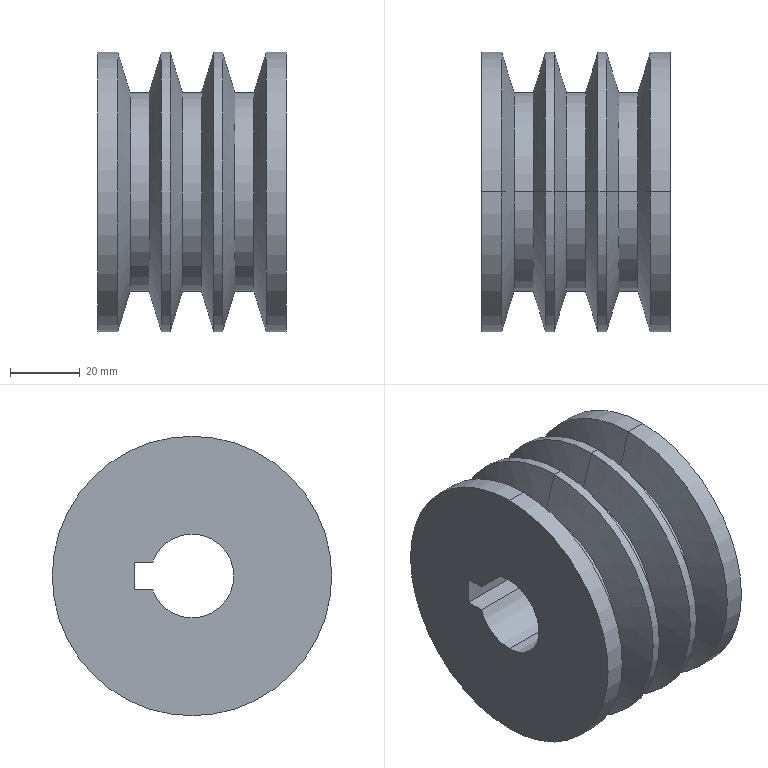Part | STEP file | Motor pulley | 1 solid | 37 faces | box 54 x 80 x 80 mm | volume 176576 mm3 | cylinder 19 | cone 12 | plane 6 | commonest cylinder face diameters 80 x8 57 x6 24 x3 2.8 x2
STEP:
#1=CARTESIAN_POINT('',(52.,-16.,1.4));
#2=VERTEX_POINT('',#1);
#3=CARTESIAN_POINT('',(52.,-16.,-1.4));
#4=VERTEX_POINT('',#3);
#5=CARTESIAN_POINT('',(52.,-16.,0.));
#6=DIRECTION('',(1.,0.,0.));
#7=DIRECTION('',(0.,0.,-1.));
#8=AXIS2_PLACEMENT_3D('',#5,#6,#7);
#9=CIRCLE('',#8,1.4);
#10=EDGE_CURVE('',#2,#4,#9,.T.);
#11=ORIENTED_EDGE('',*,*,#10,.F.);
#12=CARTESIAN_POINT('',(54.,-16.,1.4));
#13=VERTEX_POINT('',#12);
#14=CARTESIAN_POINT('',(52.,-16.,1.4));
#15=DIRECTION('',(1.,0.,0.));
#16=VECTOR('',#15,1000.);
#17=LINE('',#14,#16);
#18=EDGE_CURVE('',#2,#13,#17,.T.);
#19=ORIENTED_EDGE('',*,*,#18,.T.);
#20=CARTESIAN_POINT('',(54.,-16.,-1.4));
#21=VERTEX_POINT('',#20);
#22=CARTESIAN_POINT('',(54.,-16.,0.));
#23=DIRECTION('',(1.,0.,0.));
#24=DIRECTION('',(0.,0.,-1.));
#25=AXIS2_PLACEMENT_3D('',#22,#23,#24);
#26=CIRCLE('',#25,1.4);
#27=EDGE_CURVE('',#13,#21,#26,.T.);
#28=ORIENTED_EDGE('',*,*,#27,.T.);
#29=CARTESIAN_POINT('',(52.,-16.,-1.4));
#30=DIRECTION('',(1.,0.,0.));
#31=VECTOR('',#30,1000.);
#32=LINE('',#29,#31);
#33=EDGE_CURVE('',#4,#21,#32,.T.);
#34=ORIENTED_EDGE('',*,*,#33,.F.);
#35=EDGE_LOOP('',(#11,#19,#28,#34));
#36=FACE_OUTER_BOUND('',#35,.T.);
#37=CARTESIAN_POINT('',(52.,-16.,0.));
#38=DIRECTION('',(1.,0.,0.));
#39=DIRECTION('',(0.,0.,-1.));
#40=AXIS2_PLACEMENT_3D('',#37,#38,#39);
#41=CYLINDRICAL_SURFACE('',#40,1.4);
#42=ADVANCED_FACE('',(#36),#41,.F.);
#43=CARTESIAN_POINT('',(54.,0.,-12.));
#44=VERTEX_POINT('',#43);
#45=CARTESIAN_POINT('',(54.,0.,12.));
#46=VERTEX_POINT('',#45);
#47=CARTESIAN_POINT('',(54.,0.,0.));
#48=DIRECTION('',(-1.,0.,0.));
#49=DIRECTION('',(0.,0.,1.));
#50=AXIS2_PLACEMENT_3D('',#47,#48,#49);
#51=CIRCLE('',#50,12.);
#52=EDGE_CURVE('',#44,#46,#51,.T.);
#53=ORIENTED_EDGE('',*,*,#52,.F.);
#54=CARTESIAN_POINT('',(0.,0.,-12.));
#55=VERTEX_POINT('',#54);
#56=CARTESIAN_POINT('',(55.,0.,-12.));
#57=DIRECTION('',(-1.,0.,0.));
#58=VECTOR('',#57,1000.);
#59=LINE('',#56,#58);
#60=EDGE_CURVE('',#44,#55,#59,.T.);
#61=ORIENTED_EDGE('',*,*,#60,.T.);
#62=CARTESIAN_POINT('',(0.,0.,12.));
#63=VERTEX_POINT('',#62);
#64=CARTESIAN_POINT('',(0.,0.,0.));
#65=DIRECTION('',(-1.,0.,0.));
#66=DIRECTION('',(0.,0.,1.));
#67=AXIS2_PLACEMENT_3D('',#64,#65,#66);
#68=CIRCLE('',#67,12.);
#69=EDGE_CURVE('',#55,#63,#68,.T.);
#70=ORIENTED_EDGE('',*,*,#69,.T.);
#71=CARTESIAN_POINT('',(55.,0.,12.));
#72=DIRECTION('',(-1.,0.,0.));
#73=VECTOR('',#72,1000.);
#74=LINE('',#71,#73);
#75=EDGE_CURVE('',#46,#63,#74,.T.);
#76=ORIENTED_EDGE('',*,*,#75,.F.);
#77=EDGE_LOOP('',(#53,#61,#70,#76));
#78=FACE_OUTER_BOUND('',#77,.T.);
#79=CARTESIAN_POINT('',(55.,0.,0.));
#80=DIRECTION('',(-1.,0.,0.));
#81=DIRECTION('',(0.,0.,1.));
#82=AXIS2_PLACEMENT_3D('',#79,#80,#81);
#83=CYLINDRICAL_SURFACE('',#82,12.);
#84=ADVANCED_FACE('',(#78),#83,.F.);
#85=CARTESIAN_POINT('',(54.,11.314,4.));
#86=VERTEX_POINT('',#85);
#87=CARTESIAN_POINT('',(54.,0.,0.));
#88=DIRECTION('',(-1.,0.,0.));
#89=DIRECTION('',(0.,0.,1.));
#90=AXIS2_PLACEMENT_3D('',#87,#88,#89);
#91=CIRCLE('',#90,12.);
#92=EDGE_CURVE('',#46,#86,#91,.T.);
#93=ORIENTED_EDGE('',*,*,#92,.F.);
#94=ORIENTED_EDGE('',*,*,#75,.T.);
#95=CARTESIAN_POINT('',(0.,11.314,4.));
#96=VERTEX_POINT('',#95);
#97=CARTESIAN_POINT('',(0.,0.,0.));
#98=DIRECTION('',(-1.,0.,0.));
#99=DIRECTION('',(0.,0.,1.));
#100=AXIS2_PLACEMENT_3D('',#97,#98,#99);
#101=CIRCLE('',#100,12.);
#102=EDGE_CURVE('',#63,#96,#101,.T.);
#103=ORIENTED_EDGE('',*,*,#102,.T.);
#104=CARTESIAN_POINT('',(55.,11.314,4.));
#105=DIRECTION('',(1.,0.,0.));
#106=VECTOR('',#105,1000.);
#107=LINE('',#104,#106);
#108=EDGE_CURVE('',#96,#86,#107,.T.);
#109=ORIENTED_EDGE('',*,*,#108,.T.);
#110=EDGE_LOOP('',(#93,#94,#103,#109));
#111=FACE_OUTER_BOUND('',#110,.T.);
#112=CARTESIAN_POINT('',(55.,0.,0.));
#113=DIRECTION('',(-1.,0.,0.));
#114=DIRECTION('',(0.,0.,1.));
#115=AXIS2_PLACEMENT_3D('',#112,#113,#114);
#116=CYLINDRICAL_SURFACE('',#115,12.);
#117=ADVANCED_FACE('',(#111),#116,.F.);
#118=CARTESIAN_POINT('',(54.,0.,40.));
#119=VERTEX_POINT('',#118);
#120=CARTESIAN_POINT('',(54.,0.,-40.));
#121=VERTEX_POINT('',#120);
#122=CARTESIAN_POINT('',(54.,0.,0.));
#123=DIRECTION('',(-1.,0.,0.));
#124=DIRECTION('',(0.,0.,1.));
#125=AXIS2_PLACEMENT_3D('',#122,#123,#124);
#126=CIRCLE('',#125,40.);
#127=EDGE_CURVE('',#119,#121,#126,.T.);
#128=ORIENTED_EDGE('',*,*,#127,.T.);
#129=CARTESIAN_POINT('',(48.264,0.,-40.));
#130=VERTEX_POINT('',#129);
#131=CARTESIAN_POINT('',(0.,0.,-40.));
#132=DIRECTION('',(-1.,0.,0.));
#133=VECTOR('',#132,1000.);
#134=LINE('',#131,#133);
#135=EDGE_CURVE('',#121,#130,#134,.T.);
#136=ORIENTED_EDGE('',*,*,#135,.T.);
#137=CARTESIAN_POINT('',(48.264,0.,40.));
#138=VERTEX_POINT('',#137);
#139=CARTESIAN_POINT('',(48.264,0.,0.));
#140=DIRECTION('',(-1.,0.,0.));
#141=DIRECTION('',(0.,0.,1.));
#142=AXIS2_PLACEMENT_3D('',#139,#140,#141);
#143=CIRCLE('',#142,40.);
#144=EDGE_CURVE('',#138,#130,#143,.T.);
#145=ORIENTED_EDGE('',*,*,#144,.F.);
#146=CARTESIAN_POINT('',(0.,0.,40.));
#147=DIRECTION('',(-1.,0.,0.));
#148=VECTOR('',#147,1000.);
#149=LINE('',#146,#148);
#150=EDGE_CURVE('',#119,#138,#149,.T.);
#151=ORIENTED_EDGE('',*,*,#150,.F.);
#152=EDGE_LOOP('',(#128,#136,#145,#151));
#153=FACE_OUTER_BOUND('',#152,.T.);
#154=CARTESIAN_POINT('',(0.,0.,0.));
#155=DIRECTION('',(-1.,0.,0.));
#156=DIRECTION('',(0.,0.,1.));
#157=AXIS2_PLACEMENT_3D('',#154,#155,#156);
#158=CYLINDRICAL_SURFACE('',#157,40.);
#159=ADVANCED_FACE('',(#153),#158,.T.);
#160=CARTESIAN_POINT('',(44.748,0.,28.5));
#161=VERTEX_POINT('',#160);
#162=CARTESIAN_POINT('',(44.748,0.,-28.5));
#163=VERTEX_POINT('',#162);
#164=CARTESIAN_POINT('',(44.748,0.,0.));
#165=DIRECTION('',(-1.,0.,0.));
#166=DIRECTION('',(0.,0.,1.));
#167=AXIS2_PLACEMENT_3D('',#164,#165,#166);
#168=CIRCLE('',#167,28.5);
#169=EDGE_CURVE('',#161,#163,#168,.T.);
#170=ORIENTED_EDGE('',*,*,#169,.F.);
#171=CARTESIAN_POINT('',(48.264,0.,40.));
#172=DIRECTION('',(0.2924,0.,0.9563));
#173=VECTOR('',#172,1000.);
#174=LINE('',#171,#173);
#175=EDGE_CURVE('',#161,#138,#174,.T.);
#176=ORIENTED_EDGE('',*,*,#175,.T.);
#177=ORIENTED_EDGE('',*,*,#144,.T.);
#178=CARTESIAN_POINT('',(48.264,0.,-40.));
#179=DIRECTION('',(0.2924,0.,-0.9563));
#180=VECTOR('',#179,1000.);
#181=LINE('',#178,#180);
#182=EDGE_CURVE('',#163,#130,#181,.T.);
#183=ORIENTED_EDGE('',*,*,#182,.F.);
#184=EDGE_LOOP('',(#170,#176,#177,#183));
#185=FACE_OUTER_BOUND('',#184,.T.);
#186=CARTESIAN_POINT('',(48.264,0.,0.));
#187=DIRECTION('',(1.,0.,0.));
#188=DIRECTION('',(0.,0.,-1.));
#189=AXIS2_PLACEMENT_3D('',#186,#187,#188);
#190=CONICAL_SURFACE('',#189,40.,1.274);
#191=ADVANCED_FACE('',(#185),#190,.T.);
#192=ORIENTED_EDGE('',*,*,#169,.T.);
#193=CARTESIAN_POINT('',(39.252,0.,-28.5));
#194=VERTEX_POINT('',#193);
#195=CARTESIAN_POINT('',(0.,0.,-28.5));
#196=DIRECTION('',(-1.,0.,0.));
#197=VECTOR('',#196,1000.);
#198=LINE('',#195,#197);
#199=EDGE_CURVE('',#163,#194,#198,.T.);
#200=ORIENTED_EDGE('',*,*,#199,.T.);
#201=CARTESIAN_POINT('',(39.252,0.,28.5));
#202=VERTEX_POINT('',#201);
#203=CARTESIAN_POINT('',(39.252,0.,0.));
#204=DIRECTION('',(-1.,0.,0.));
#205=DIRECTION('',(0.,0.,1.));
#206=AXIS2_PLACEMENT_3D('',#203,#204,#205);
#207=CIRCLE('',#206,28.5);
#208=EDGE_CURVE('',#202,#194,#207,.T.);
#209=ORIENTED_EDGE('',*,*,#208,.F.);
#210=CARTESIAN_POINT('',(0.,0.,28.5));
#211=DIRECTION('',(-1.,0.,0.));
#212=VECTOR('',#211,1000.);
#213=LINE('',#210,#212);
#214=EDGE_CURVE('',#161,#202,#213,.T.);
#215=ORIENTED_EDGE('',*,*,#214,.F.);
#216=EDGE_LOOP('',(#192,#200,#209,#215));
#217=FACE_OUTER_BOUND('',#216,.T.);
#218=CARTESIAN_POINT('',(0.,0.,0.));
#219=DIRECTION('',(-1.,0.,0.));
#220=DIRECTION('',(0.,0.,1.));
#221=AXIS2_PLACEMENT_3D('',#218,#219,#220);
#222=CYLINDRICAL_SURFACE('',#221,28.5);
#223=ADVANCED_FACE('',(#217),#222,.T.);
#224=ORIENTED_EDGE('',*,*,#208,.T.);
#225=CARTESIAN_POINT('',(35.736,0.,-40.));
#226=VERTEX_POINT('',#225);
#227=CARTESIAN_POINT('',(39.252,0.,-28.5));
#228=DIRECTION('',(-0.2924,0.,-0.9563));
#229=VECTOR('',#228,1000.);
#230=LINE('',#227,#229);
#231=EDGE_CURVE('',#194,#226,#230,.T.);
#232=ORIENTED_EDGE('',*,*,#231,.T.);
#233=CARTESIAN_POINT('',(35.736,0.,40.));
#234=VERTEX_POINT('',#233);
#235=CARTESIAN_POINT('',(35.736,0.,0.));
#236=DIRECTION('',(-1.,0.,0.));
#237=DIRECTION('',(0.,0.,1.));
#238=AXIS2_PLACEMENT_3D('',#235,#236,#237);
#239=CIRCLE('',#238,40.);
#240=EDGE_CURVE('',#234,#226,#239,.T.);
#241=ORIENTED_EDGE('',*,*,#240,.F.);
#242=CARTESIAN_POINT('',(39.252,0.,28.5));
#243=DIRECTION('',(-0.2924,0.,0.9563));
#244=VECTOR('',#243,1000.);
#245=LINE('',#242,#244);
#246=EDGE_CURVE('',#202,#234,#245,.T.);
#247=ORIENTED_EDGE('',*,*,#246,.F.);
#248=EDGE_LOOP('',(#224,#232,#241,#247));
#249=FACE_OUTER_BOUND('',#248,.T.);
#250=CARTESIAN_POINT('',(39.252,0.,0.));
#251=DIRECTION('',(-1.,0.,0.));
#252=DIRECTION('',(0.,0.,1.));
#253=AXIS2_PLACEMENT_3D('',#250,#251,#252);
#254=CONICAL_SURFACE('',#253,28.5,1.274);
#255=ADVANCED_FACE('',(#249),#254,.T.);
#256=ORIENTED_EDGE('',*,*,#240,.T.);
#257=CARTESIAN_POINT('',(33.264,0.,-40.));
#258=VERTEX_POINT('',#257);
#259=CARTESIAN_POINT('',(0.,0.,-40.));
#260=DIRECTION('',(-1.,0.,0.));
#261=VECTOR('',#260,1000.);
#262=LINE('',#259,#261);
#263=EDGE_CURVE('',#226,#258,#262,.T.);
#264=ORIENTED_EDGE('',*,*,#263,.T.);
#265=CARTESIAN_POINT('',(33.264,0.,40.));
#266=VERTEX_POINT('',#265);
#267=CARTESIAN_POINT('',(33.264,0.,0.));
#268=DIRECTION('',(-1.,0.,0.));
#269=DIRECTION('',(0.,0.,1.));
#270=AXIS2_PLACEMENT_3D('',#267,#268,#269);
#271=CIRCLE('',#270,40.);
#272=EDGE_CURVE('',#266,#258,#271,.T.);
#273=ORIENTED_EDGE('',*,*,#272,.F.);
#274=CARTESIAN_POINT('',(0.,0.,40.));
#275=DIRECTION('',(-1.,0.,0.));
#276=VECTOR('',#275,1000.);
#277=LINE('',#274,#276);
#278=EDGE_CURVE('',#234,#266,#277,.T.);
#279=ORIENTED_EDGE('',*,*,#278,.F.);
#280=EDGE_LOOP('',(#256,#264,#273,#279));
#281=FACE_OUTER_BOUND('',#280,.T.);
#282=CARTESIAN_POINT('',(0.,0.,0.));
#283=DIRECTION('',(-1.,0.,0.));
#284=DIRECTION('',(0.,0.,1.));
#285=AXIS2_PLACEMENT_3D('',#282,#283,#284);
#286=CYLINDRICAL_SURFACE('',#285,40.);
#287=ADVANCED_FACE('',(#281),#286,.T.);
#288=CARTESIAN_POINT('',(29.748,0.,28.5));
#289=VERTEX_POINT('',#288);
#290=CARTESIAN_POINT('',(29.748,0.,-28.5));
#291=VERTEX_POINT('',#290);
#292=CARTESIAN_POINT('',(29.748,0.,0.));
#293=DIRECTION('',(-1.,0.,0.));
#294=DIRECTION('',(0.,0.,1.));
#295=AXIS2_PLACEMENT_3D('',#292,#293,#294);
#296=CIRCLE('',#295,28.5);
#297=EDGE_CURVE('',#289,#291,#296,.T.);
#298=ORIENTED_EDGE('',*,*,#297,.F.);
#299=CARTESIAN_POINT('',(33.264,0.,40.));
#300=DIRECTION('',(0.2924,0.,0.9563));
#301=VECTOR('',#300,1000.);
#302=LINE('',#299,#301);
#303=EDGE_CURVE('',#289,#266,#302,.T.);
#304=ORIENTED_EDGE('',*,*,#303,.T.);
#305=ORIENTED_EDGE('',*,*,#272,.T.);
#306=CARTESIAN_POINT('',(33.264,0.,-40.));
#307=DIRECTION('',(0.2924,0.,-0.9563));
#308=VECTOR('',#307,1000.);
#309=LINE('',#306,#308);
#310=EDGE_CURVE('',#291,#258,#309,.T.);
#311=ORIENTED_EDGE('',*,*,#310,.F.);
#312=EDGE_LOOP('',(#298,#304,#305,#311));
#313=FACE_OUTER_BOUND('',#312,.T.);
#314=CARTESIAN_POINT('',(33.264,0.,0.));
#315=DIRECTION('',(1.,0.,0.));
#316=DIRECTION('',(0.,0.,-1.));
#317=AXIS2_PLACEMENT_3D('',#314,#315,#316);
#318=CONICAL_SURFACE('',#317,40.,1.274);
#319=ADVANCED_FACE('',(#313),#318,.T.);
#320=ORIENTED_EDGE('',*,*,#297,.T.);
#321=CARTESIAN_POINT('',(24.252,0.,-28.5));
#322=VERTEX_POINT('',#321);
#323=CARTESIAN_POINT('',(0.,0.,-28.5));
#324=DIRECTION('',(-1.,0.,0.));
#325=VECTOR('',#324,1000.);
#326=LINE('',#323,#325);
#327=EDGE_CURVE('',#291,#322,#326,.T.);
#328=ORIENTED_EDGE('',*,*,#327,.T.);
#329=CARTESIAN_POINT('',(24.252,0.,28.5));
#330=VERTEX_POINT('',#329);
#331=CARTESIAN_POINT('',(24.252,0.,0.));
#332=DIRECTION('',(-1.,0.,0.));
#333=DIRECTION('',(0.,0.,1.));
#334=AXIS2_PLACEMENT_3D('',#331,#332,#333);
#335=CIRCLE('',#334,28.5);
#336=EDGE_CURVE('',#330,#322,#335,.T.);
#337=ORIENTED_EDGE('',*,*,#336,.F.);
#338=CARTESIAN_POINT('',(0.,0.,28.5));
#339=DIRECTION('',(-1.,0.,0.));
#340=VECTOR('',#339,1000.);
#341=LINE('',#338,#340);
#342=EDGE_CURVE('',#289,#330,#341,.T.);
#343=ORIENTED_EDGE('',*,*,#342,.F.);
#344=EDGE_LOOP('',(#320,#328,#337,#343));
#345=FACE_OUTER_BOUND('',#344,.T.);
#346=CARTESIAN_POINT('',(0.,0.,0.));
#347=DIRECTION('',(-1.,0.,0.));
#348=DIRECTION('',(0.,0.,1.));
#349=AXIS2_PLACEMENT_3D('',#346,#347,#348);
#350=CYLINDRICAL_SURFACE('',#349,28.5);
#351=ADVANCED_FACE('',(#345),#350,.T.);
#352=ORIENTED_EDGE('',*,*,#336,.T.);
#353=CARTESIAN_POINT('',(20.736,0.,-40.));
#354=VERTEX_POINT('',#353);
#355=CARTESIAN_POINT('',(24.252,0.,-28.5));
#356=DIRECTION('',(-0.2924,0.,-0.9563));
#357=VECTOR('',#356,1000.);
#358=LINE('',#355,#357);
#359=EDGE_CURVE('',#322,#354,#358,.T.);
#360=ORIENTED_EDGE('',*,*,#359,.T.);
#361=CARTESIAN_POINT('',(20.736,0.,40.));
#362=VERTEX_POINT('',#361);
#363=CARTESIAN_POINT('',(20.736,0.,0.));
#364=DIRECTION('',(-1.,0.,0.));
#365=DIRECTION('',(0.,0.,1.));
#366=AXIS2_PLACEMENT_3D('',#363,#364,#365);
#367=CIRCLE('',#366,40.);
#368=EDGE_CURVE('',#362,#354,#367,.T.);
#369=ORIENTED_EDGE('',*,*,#368,.F.);
#370=CARTESIAN_POINT('',(24.252,0.,28.5));
#371=DIRECTION('',(-0.2924,0.,0.9563));
#372=VECTOR('',#371,1000.);
#373=LINE('',#370,#372);
#374=EDGE_CURVE('',#330,#362,#373,.T.);
#375=ORIENTED_EDGE('',*,*,#374,.F.);
#376=EDGE_LOOP('',(#352,#360,#369,#375));
#377=FACE_OUTER_BOUND('',#376,.T.);
#378=CARTESIAN_POINT('',(24.252,0.,0.));
#379=DIRECTION('',(-1.,0.,0.));
#380=DIRECTION('',(0.,0.,1.));
#381=AXIS2_PLACEMENT_3D('',#378,#379,#380);
#382=CONICAL_SURFACE('',#381,28.5,1.274);
#383=ADVANCED_FACE('',(#377),#382,.T.);
#384=ORIENTED_EDGE('',*,*,#368,.T.);
#385=CARTESIAN_POINT('',(18.264,0.,-40.));
#386=VERTEX_POINT('',#385);
#387=CARTESIAN_POINT('',(0.,0.,-40.));
#388=DIRECTION('',(-1.,0.,0.));
#389=VECTOR('',#388,1000.);
#390=LINE('',#387,#389);
#391=EDGE_CURVE('',#354,#386,#390,.T.);
#392=ORIENTED_EDGE('',*,*,#391,.T.);
#393=CARTESIAN_POINT('',(18.264,0.,40.));
#394=VERTEX_POINT('',#393);
#395=CARTESIAN_POINT('',(18.264,0.,0.));
#396=DIRECTION('',(-1.,0.,0.));
#397=DIRECTION('',(0.,0.,1.));
#398=AXIS2_PLACEMENT_3D('',#395,#396,#397);
#399=CIRCLE('',#398,40.);
#400=EDGE_CURVE('',#394,#386,#399,.T.);
#401=ORIENTED_EDGE('',*,*,#400,.F.);
#402=CARTESIAN_POINT('',(0.,0.,40.));
#403=DIRECTION('',(-1.,0.,0.));
#404=VECTOR('',#403,1000.);
#405=LINE('',#402,#404);
#406=EDGE_CURVE('',#362,#394,#405,.T.);
#407=ORIENTED_EDGE('',*,*,#406,.F.);
#408=EDGE_LOOP('',(#384,#392,#401,#407));
#409=FACE_OUTER_BOUND('',#408,.T.);
#410=CARTESIAN_POINT('',(0.,0.,0.));
#411=DIRECTION('',(-1.,0.,0.));
#412=DIRECTION('',(0.,0.,1.));
#413=AXIS2_PLACEMENT_3D('',#410,#411,#412);
#414=CYLINDRICAL_SURFACE('',#413,40.);
#415=ADVANCED_FACE('',(#409),#414,.T.);
#416=CARTESIAN_POINT('',(14.748,0.,28.5));
#417=VERTEX_POINT('',#416);
#418=CARTESIAN_POINT('',(14.748,0.,-28.5));
#419=VERTEX_POINT('',#418);
#420=CARTESIAN_POINT('',(14.748,0.,0.));
#421=DIRECTION('',(-1.,0.,0.));
#422=DIRECTION('',(0.,0.,1.));
#423=AXIS2_PLACEMENT_3D('',#420,#421,#422);
#424=CIRCLE('',#423,28.5);
#425=EDGE_CURVE('',#417,#419,#424,.T.);
#426=ORIENTED_EDGE('',*,*,#425,.F.);
#427=CARTESIAN_POINT('',(18.264,0.,40.));
#428=DIRECTION('',(0.2924,0.,0.9563));
#429=VECTOR('',#428,1000.);
#430=LINE('',#427,#429);
#431=EDGE_CURVE('',#417,#394,#430,.T.);
#432=ORIENTED_EDGE('',*,*,#431,.T.);
#433=ORIENTED_EDGE('',*,*,#400,.T.);
#434=CARTESIAN_POINT('',(18.264,0.,-40.));
#435=DIRECTION('',(0.2924,0.,-0.9563));
#436=VECTOR('',#435,1000.);
#437=LINE('',#434,#436);
#438=EDGE_CURVE('',#419,#386,#437,.T.);
#439=ORIENTED_EDGE('',*,*,#438,.F.);
#440=EDGE_LOOP('',(#426,#432,#433,#439));
#441=FACE_OUTER_BOUND('',#440,.T.);
#442=CARTESIAN_POINT('',(18.264,0.,0.));
#443=DIRECTION('',(1.,0.,0.));
#444=DIRECTION('',(0.,0.,-1.));
#445=AXIS2_PLACEMENT_3D('',#442,#443,#444);
#446=CONICAL_SURFACE('',#445,40.,1.274);
#447=ADVANCED_FACE('',(#441),#446,.T.);
#448=ORIENTED_EDGE('',*,*,#425,.T.);
#449=CARTESIAN_POINT('',(9.252,0.,-28.5));
#450=VERTEX_POINT('',#449);
#451=CARTESIAN_POINT('',(0.,0.,-28.5));
#452=DIRECTION('',(-1.,0.,0.));
#453=VECTOR('',#452,1000.);
#454=LINE('',#451,#453);
#455=EDGE_CURVE('',#419,#450,#454,.T.);
#456=ORIENTED_EDGE('',*,*,#455,.T.);
#457=CARTESIAN_POINT('',(9.252,0.,28.5));
#458=VERTEX_POINT('',#457);
#459=CARTESIAN_POINT('',(9.252,0.,0.));
#460=DIRECTION('',(-1.,0.,0.));
#461=DIRECTION('',(0.,0.,1.));
#462=AXIS2_PLACEMENT_3D('',#459,#460,#461);
#463=CIRCLE('',#462,28.5);
#464=EDGE_CURVE('',#458,#450,#463,.T.);
#465=ORIENTED_EDGE('',*,*,#464,.F.);
#466=CARTESIAN_POINT('',(0.,0.,28.5));
#467=DIRECTION('',(-1.,0.,0.));
#468=VECTOR('',#467,1000.);
#469=LINE('',#466,#468);
#470=EDGE_CURVE('',#417,#458,#469,.T.);
#471=ORIENTED_EDGE('',*,*,#470,.F.);
#472=EDGE_LOOP('',(#448,#456,#465,#471));
#473=FACE_OUTER_BOUND('',#472,.T.);
#474=CARTESIAN_POINT('',(0.,0.,0.));
#475=DIRECTION('',(-1.,0.,0.));
#476=DIRECTION('',(0.,0.,1.));
#477=AXIS2_PLACEMENT_3D('',#474,#475,#476);
#478=CYLINDRICAL_SURFACE('',#477,28.5);
#479=ADVANCED_FACE('',(#473),#478,.T.);
#480=ORIENTED_EDGE('',*,*,#464,.T.);
#481=CARTESIAN_POINT('',(5.736,0.,-40.));
#482=VERTEX_POINT('',#481);
#483=CARTESIAN_POINT('',(9.252,0.,-28.5));
#484=DIRECTION('',(-0.2924,0.,-0.9563));
#485=VECTOR('',#484,1000.);
#486=LINE('',#483,#485);
#487=EDGE_CURVE('',#450,#482,#486,.T.);
#488=ORIENTED_EDGE('',*,*,#487,.T.);
#489=CARTESIAN_POINT('',(5.736,0.,40.));
#490=VERTEX_POINT('',#489);
#491=CARTESIAN_POINT('',(5.736,0.,0.));
#492=DIRECTION('',(-1.,0.,0.));
#493=DIRECTION('',(0.,0.,1.));
#494=AXIS2_PLACEMENT_3D('',#491,#492,#493);
#495=CIRCLE('',#494,40.);
#496=EDGE_CURVE('',#490,#482,#495,.T.);
#497=ORIENTED_EDGE('',*,*,#496,.F.);
#498=CARTESIAN_POINT('',(9.252,0.,28.5));
#499=DIRECTION('',(-0.2924,0.,0.9563));
#500=VECTOR('',#499,1000.);
#501=LINE('',#498,#500);
#502=EDGE_CURVE('',#458,#490,#501,.T.);
#503=ORIENTED_EDGE('',*,*,#502,.F.);
#504=EDGE_LOOP('',(#480,#488,#497,#503));
#505=FACE_OUTER_BOUND('',#504,.T.);
#506=CARTESIAN_POINT('',(9.252,0.,0.));
#507=DIRECTION('',(-1.,0.,0.));
#508=DIRECTION('',(0.,0.,1.));
#509=AXIS2_PLACEMENT_3D('',#506,#507,#508);
#510=CONICAL_SURFACE('',#509,28.5,1.274);
#511=ADVANCED_FACE('',(#505),#510,.T.);
#512=ORIENTED_EDGE('',*,*,#496,.T.);
#513=CARTESIAN_POINT('',(0.,0.,-40.));
#514=VERTEX_POINT('',#513);
#515=CARTESIAN_POINT('',(0.,0.,-40.));
#516=DIRECTION('',(-1.,0.,0.));
#517=VECTOR('',#516,1000.);
#518=LINE('',#515,#517);
#519=EDGE_CURVE('',#482,#514,#518,.T.);
#520=ORIENTED_EDGE('',*,*,#519,.T.);
#521=CARTESIAN_POINT('',(0.,0.,40.));
#522=VERTEX_POINT('',#521);
#523=CARTESIAN_POINT('',(0.,0.,0.));
#524=DIRECTION('',(-1.,0.,0.));
#525=DIRECTION('',(0.,0.,1.));
#526=AXIS2_PLACEMENT_3D('',#523,#524,#525);
#527=CIRCLE('',#526,40.);
#528=EDGE_CURVE('',#522,#514,#527,.T.);
#529=ORIENTED_EDGE('',*,*,#528,.F.);
#530=CARTESIAN_POINT('',(0.,0.,40.));
#531=DIRECTION('',(-1.,0.,0.));
#532=VECTOR('',#531,1000.);
#533=LINE('',#530,#532);
#534=EDGE_CURVE('',#490,#522,#533,.T.);
#535=ORIENTED_EDGE('',*,*,#534,.F.);
#536=EDGE_LOOP('',(#512,#520,#529,#535));
#537=FACE_OUTER_BOUND('',#536,.T.);
#538=CARTESIAN_POINT('',(0.,0.,0.));
#539=DIRECTION('',(-1.,0.,0.));
#540=DIRECTION('',(0.,0.,1.));
#541=AXIS2_PLACEMENT_3D('',#538,#539,#540);
#542=CYLINDRICAL_SURFACE('',#541,40.);
#543=ADVANCED_FACE('',(#537),#542,.T.);
#544=CARTESIAN_POINT('',(0.,16.5,4.));
#545=VERTEX_POINT('',#544);
#546=CARTESIAN_POINT('',(0.,16.5,-4.));
#547=VERTEX_POINT('',#546);
#548=CARTESIAN_POINT('',(0.,16.5,-4.));
#549=DIRECTION('',(0.,0.,-1.));
#550=VECTOR('',#549,1000.);
#551=LINE('',#548,#550);
#552=EDGE_CURVE('',#545,#547,#551,.T.);
#553=ORIENTED_EDGE('',*,*,#552,.F.);
#554=CARTESIAN_POINT('',(0.,16.5,4.));
#555=DIRECTION('',(0.,1.,0.));
#556=VECTOR('',#555,1000.);
#557=LINE('',#554,#556);
#558=EDGE_CURVE('',#96,#545,#557,.T.);
#559=ORIENTED_EDGE('',*,*,#558,.F.);
#560=ORIENTED_EDGE('',*,*,#102,.F.);
#561=ORIENTED_EDGE('',*,*,#69,.F.);
#562=CARTESIAN_POINT('',(0.,11.314,-4.));
#563=VERTEX_POINT('',#562);
#564=CARTESIAN_POINT('',(0.,0.,0.));
#565=DIRECTION('',(-1.,0.,0.));
#566=DIRECTION('',(0.,0.,1.));
#567=AXIS2_PLACEMENT_3D('',#564,#565,#566);
#568=CIRCLE('',#567,12.);
#569=EDGE_CURVE('',#563,#55,#568,.T.);
#570=ORIENTED_EDGE('',*,*,#569,.F.);
#571=CARTESIAN_POINT('',(0.,16.5,-4.));
#572=DIRECTION('',(0.,-1.,0.));
#573=VECTOR('',#572,1000.);
#574=LINE('',#571,#573);
#575=EDGE_CURVE('',#547,#563,#574,.T.);
#576=ORIENTED_EDGE('',*,*,#575,.F.);
#577=EDGE_LOOP('',(#553,#559,#560,#561,#570,#576));
#578=FACE_BOUND('',#577,.T.);
#579=ORIENTED_EDGE('',*,*,#528,.T.);
#580=CARTESIAN_POINT('',(0.,0.,0.));
#581=DIRECTION('',(-1.,0.,0.));
#582=DIRECTION('',(0.,0.,1.));
#583=AXIS2_PLACEMENT_3D('',#580,#581,#582);
#584=CIRCLE('',#583,40.);
#585=EDGE_CURVE('',#514,#522,#584,.T.);
#586=ORIENTED_EDGE('',*,*,#585,.T.);
#587=EDGE_LOOP('',(#579,#586));
#588=FACE_OUTER_BOUND('',#587,.T.);
#589=CARTESIAN_POINT('',(0.,37.5,0.));
#590=DIRECTION('',(1.,0.,0.));
#591=DIRECTION('',(0.,0.,-1.));
#592=AXIS2_PLACEMENT_3D('',#589,#590,#591);
#593=PLANE('',#592);
#594=ADVANCED_FACE('',(#578,#588),#593,.F.);
#595=ORIENTED_EDGE('',*,*,#519,.F.);
#596=CARTESIAN_POINT('',(5.736,0.,0.));
#597=DIRECTION('',(-1.,0.,0.));
#598=DIRECTION('',(0.,0.,1.));
#599=AXIS2_PLACEMENT_3D('',#596,#597,#598);
#600=CIRCLE('',#599,40.);
#601=EDGE_CURVE('',#482,#490,#600,.T.);
#602=ORIENTED_EDGE('',*,*,#601,.T.);
#603=ORIENTED_EDGE('',*,*,#534,.T.);
#604=ORIENTED_EDGE('',*,*,#585,.F.);
#605=EDGE_LOOP('',(#595,#602,#603,#604));
#606=FACE_OUTER_BOUND('',#605,.T.);
#607=CARTESIAN_POINT('',(0.,0.,0.));
#608=DIRECTION('',(-1.,0.,0.));
#609=DIRECTION('',(0.,0.,1.));
#610=AXIS2_PLACEMENT_3D('',#607,#608,#609);
#611=CYLINDRICAL_SURFACE('',#610,40.);
#612=ADVANCED_FACE('',(#606),#611,.T.);
#613=ORIENTED_EDGE('',*,*,#487,.F.);
#614=CARTESIAN_POINT('',(9.252,0.,0.));
#615=DIRECTION('',(-1.,0.,0.));
#616=DIRECTION('',(0.,0.,1.));
#617=AXIS2_PLACEMENT_3D('',#614,#615,#616);
#618=CIRCLE('',#617,28.5);
#619=EDGE_CURVE('',#450,#458,#618,.T.);
#620=ORIENTED_EDGE('',*,*,#619,.T.);
#621=ORIENTED_EDGE('',*,*,#502,.T.);
#622=ORIENTED_EDGE('',*,*,#601,.F.);
#623=EDGE_LOOP('',(#613,#620,#621,#622));
#624=FACE_OUTER_BOUND('',#623,.T.);
#625=CARTESIAN_POINT('',(9.252,0.,0.));
#626=DIRECTION('',(-1.,0.,0.));
#627=DIRECTION('',(0.,0.,1.));
#628=AXIS2_PLACEMENT_3D('',#625,#626,#627);
#629=CONICAL_SURFACE('',#628,28.5,1.274);
#630=ADVANCED_FACE('',(#624),#629,.T.);
#631=ORIENTED_EDGE('',*,*,#455,.F.);
#632=CARTESIAN_POINT('',(14.748,0.,0.));
#633=DIRECTION('',(-1.,0.,0.));
#634=DIRECTION('',(0.,0.,1.));
#635=AXIS2_PLACEMENT_3D('',#632,#633,#634);
#636=CIRCLE('',#635,28.5);
#637=EDGE_CURVE('',#419,#417,#636,.T.);
#638=ORIENTED_EDGE('',*,*,#637,.T.);
#639=ORIENTED_EDGE('',*,*,#470,.T.);
#640=ORIENTED_EDGE('',*,*,#619,.F.);
#641=EDGE_LOOP('',(#631,#638,#639,#640));
#642=FACE_OUTER_BOUND('',#641,.T.);
#643=CARTESIAN_POINT('',(0.,0.,0.));
#644=DIRECTION('',(-1.,0.,0.));
#645=DIRECTION('',(0.,0.,1.));
#646=AXIS2_PLACEMENT_3D('',#643,#644,#645);
#647=CYLINDRICAL_SURFACE('',#646,28.5);
#648=ADVANCED_FACE('',(#642),#647,.T.);
#649=ORIENTED_EDGE('',*,*,#431,.F.);
#650=ORIENTED_EDGE('',*,*,#637,.F.);
#651=ORIENTED_EDGE('',*,*,#438,.T.);
#652=CARTESIAN_POINT('',(18.264,0.,0.));
#653=DIRECTION('',(-1.,0.,0.));
#654=DIRECTION('',(0.,0.,1.));
#655=AXIS2_PLACEMENT_3D('',#652,#653,#654);
#656=CIRCLE('',#655,40.);
#657=EDGE_CURVE('',#386,#394,#656,.T.);
#658=ORIENTED_EDGE('',*,*,#657,.T.);
#659=EDGE_LOOP('',(#649,#650,#651,#658));
#660=FACE_OUTER_BOUND('',#659,.T.);
#661=CARTESIAN_POINT('',(18.264,0.,0.));
#662=DIRECTION('',(1.,0.,0.));
#663=DIRECTION('',(0.,0.,-1.));
#664=AXIS2_PLACEMENT_3D('',#661,#662,#663);
#665=CONICAL_SURFACE('',#664,40.,1.274);
#666=ADVANCED_FACE('',(#660),#665,.T.);
#667=ORIENTED_EDGE('',*,*,#391,.F.);
#668=CARTESIAN_POINT('',(20.736,0.,0.));
#669=DIRECTION('',(-1.,0.,0.));
#670=DIRECTION('',(0.,0.,1.));
#671=AXIS2_PLACEMENT_3D('',#668,#669,#670);
#672=CIRCLE('',#671,40.);
#673=EDGE_CURVE('',#354,#362,#672,.T.);
#674=ORIENTED_EDGE('',*,*,#673,.T.);
#675=ORIENTED_EDGE('',*,*,#406,.T.);
#676=ORIENTED_EDGE('',*,*,#657,.F.);
#677=EDGE_LOOP('',(#667,#674,#675,#676));
#678=FACE_OUTER_BOUND('',#677,.T.);
#679=CARTESIAN_POINT('',(0.,0.,0.));
#680=DIRECTION('',(-1.,0.,0.));
#681=DIRECTION('',(0.,0.,1.));
#682=AXIS2_PLACEMENT_3D('',#679,#680,#681);
#683=CYLINDRICAL_SURFACE('',#682,40.);
#684=ADVANCED_FACE('',(#678),#683,.T.);
#685=ORIENTED_EDGE('',*,*,#359,.F.);
#686=CARTESIAN_POINT('',(24.252,0.,0.));
#687=DIRECTION('',(-1.,0.,0.));
#688=DIRECTION('',(0.,0.,1.));
#689=AXIS2_PLACEMENT_3D('',#686,#687,#688);
#690=CIRCLE('',#689,28.5);
#691=EDGE_CURVE('',#322,#330,#690,.T.);
#692=ORIENTED_EDGE('',*,*,#691,.T.);
#693=ORIENTED_EDGE('',*,*,#374,.T.);
#694=ORIENTED_EDGE('',*,*,#673,.F.);
#695=EDGE_LOOP('',(#685,#692,#693,#694));
#696=FACE_OUTER_BOUND('',#695,.T.);
#697=CARTESIAN_POINT('',(24.252,0.,0.));
#698=DIRECTION('',(-1.,0.,0.));
#699=DIRECTION('',(0.,0.,1.));
#700=AXIS2_PLACEMENT_3D('',#697,#698,#699);
#701=CONICAL_SURFACE('',#700,28.5,1.274);
#702=ADVANCED_FACE('',(#696),#701,.T.);
#703=ORIENTED_EDGE('',*,*,#327,.F.);
#704=CARTESIAN_POINT('',(29.748,0.,0.));
#705=DIRECTION('',(-1.,0.,0.));
#706=DIRECTION('',(0.,0.,1.));
#707=AXIS2_PLACEMENT_3D('',#704,#705,#706);
#708=CIRCLE('',#707,28.5);
#709=EDGE_CURVE('',#291,#289,#708,.T.);
#710=ORIENTED_EDGE('',*,*,#709,.T.);
#711=ORIENTED_EDGE('',*,*,#342,.T.);
#712=ORIENTED_EDGE('',*,*,#691,.F.);
#713=EDGE_LOOP('',(#703,#710,#711,#712));
#714=FACE_OUTER_BOUND('',#713,.T.);
#715=CARTESIAN_POINT('',(0.,0.,0.));
#716=DIRECTION('',(-1.,0.,0.));
#717=DIRECTION('',(0.,0.,1.));
#718=AXIS2_PLACEMENT_3D('',#715,#716,#717);
#719=CYLINDRICAL_SURFACE('',#718,28.5);
#720=ADVANCED_FACE('',(#714),#719,.T.);
#721=ORIENTED_EDGE('',*,*,#303,.F.);
#722=ORIENTED_EDGE('',*,*,#709,.F.);
#723=ORIENTED_EDGE('',*,*,#310,.T.);
#724=CARTESIAN_POINT('',(33.264,0.,0.));
#725=DIRECTION('',(-1.,0.,0.));
#726=DIRECTION('',(0.,0.,1.));
#727=AXIS2_PLACEMENT_3D('',#724,#725,#726);
#728=CIRCLE('',#727,40.);
#729=EDGE_CURVE('',#258,#266,#728,.T.);
#730=ORIENTED_EDGE('',*,*,#729,.T.);
#731=EDGE_LOOP('',(#721,#722,#723,#730));
#732=FACE_OUTER_BOUND('',#731,.T.);
#733=CARTESIAN_POINT('',(33.264,0.,0.));
#734=DIRECTION('',(1.,0.,0.));
#735=DIRECTION('',(0.,0.,-1.));
#736=AXIS2_PLACEMENT_3D('',#733,#734,#735);
#737=CONICAL_SURFACE('',#736,40.,1.274);
#738=ADVANCED_FACE('',(#732),#737,.T.);
#739=ORIENTED_EDGE('',*,*,#263,.F.);
#740=CARTESIAN_POINT('',(35.736,0.,0.));
#741=DIRECTION('',(-1.,0.,0.));
#742=DIRECTION('',(0.,0.,1.));
#743=AXIS2_PLACEMENT_3D('',#740,#741,#742);
#744=CIRCLE('',#743,40.);
#745=EDGE_CURVE('',#226,#234,#744,.T.);
#746=ORIENTED_EDGE('',*,*,#745,.T.);
#747=ORIENTED_EDGE('',*,*,#278,.T.);
#748=ORIENTED_EDGE('',*,*,#729,.F.);
#749=EDGE_LOOP('',(#739,#746,#747,#748));
#750=FACE_OUTER_BOUND('',#749,.T.);
#751=CARTESIAN_POINT('',(0.,0.,0.));
#752=DIRECTION('',(-1.,0.,0.));
#753=DIRECTION('',(0.,0.,1.));
#754=AXIS2_PLACEMENT_3D('',#751,#752,#753);
#755=CYLINDRICAL_SURFACE('',#754,40.);
#756=ADVANCED_FACE('',(#750),#755,.T.);
#757=ORIENTED_EDGE('',*,*,#231,.F.);
#758=CARTESIAN_POINT('',(39.252,0.,0.));
#759=DIRECTION('',(-1.,0.,0.));
#760=DIRECTION('',(0.,0.,1.));
#761=AXIS2_PLACEMENT_3D('',#758,#759,#760);
#762=CIRCLE('',#761,28.5);
#763=EDGE_CURVE('',#194,#202,#762,.T.);
#764=ORIENTED_EDGE('',*,*,#763,.T.);
#765=ORIENTED_EDGE('',*,*,#246,.T.);
#766=ORIENTED_EDGE('',*,*,#745,.F.);
#767=EDGE_LOOP('',(#757,#764,#765,#766));
#768=FACE_OUTER_BOUND('',#767,.T.);
#769=CARTESIAN_POINT('',(39.252,0.,0.));
#770=DIRECTION('',(-1.,0.,0.));
#771=DIRECTION('',(0.,0.,1.));
#772=AXIS2_PLACEMENT_3D('',#769,#770,#771);
#773=CONICAL_SURFACE('',#772,28.5,1.274);
#774=ADVANCED_FACE('',(#768),#773,.T.);
#775=ORIENTED_EDGE('',*,*,#199,.F.);
#776=CARTESIAN_POINT('',(44.748,0.,0.));
#777=DIRECTION('',(-1.,0.,0.));
#778=DIRECTION('',(0.,0.,1.));
#779=AXIS2_PLACEMENT_3D('',#776,#777,#778);
#780=CIRCLE('',#779,28.5);
#781=EDGE_CURVE('',#163,#161,#780,.T.);
#782=ORIENTED_EDGE('',*,*,#781,.T.);
#783=ORIENTED_EDGE('',*,*,#214,.T.);
#784=ORIENTED_EDGE('',*,*,#763,.F.);
#785=EDGE_LOOP('',(#775,#782,#783,#784));
#786=FACE_OUTER_BOUND('',#785,.T.);
#787=CARTESIAN_POINT('',(0.,0.,0.));
#788=DIRECTION('',(-1.,0.,0.));
#789=DIRECTION('',(0.,0.,1.));
#790=AXIS2_PLACEMENT_3D('',#787,#788,#789);
#791=CYLINDRICAL_SURFACE('',#790,28.5);
#792=ADVANCED_FACE('',(#786),#791,.T.);
#793=ORIENTED_EDGE('',*,*,#175,.F.);
#794=ORIENTED_EDGE('',*,*,#781,.F.);
#795=ORIENTED_EDGE('',*,*,#182,.T.);
#796=CARTESIAN_POINT('',(48.264,0.,0.));
#797=DIRECTION('',(-1.,0.,0.));
#798=DIRECTION('',(0.,0.,1.));
#799=AXIS2_PLACEMENT_3D('',#796,#797,#798);
#800=CIRCLE('',#799,40.);
#801=EDGE_CURVE('',#130,#138,#800,.T.);
#802=ORIENTED_EDGE('',*,*,#801,.T.);
#803=EDGE_LOOP('',(#793,#794,#795,#802));
#804=FACE_OUTER_BOUND('',#803,.T.);
#805=CARTESIAN_POINT('',(48.264,0.,0.));
#806=DIRECTION('',(1.,0.,0.));
#807=DIRECTION('',(0.,0.,-1.));
#808=AXIS2_PLACEMENT_3D('',#805,#806,#807);
#809=CONICAL_SURFACE('',#808,40.,1.274);
#810=ADVANCED_FACE('',(#804),#809,.T.);
#811=ORIENTED_EDGE('',*,*,#135,.F.);
#812=CARTESIAN_POINT('',(54.,0.,0.));
#813=DIRECTION('',(-1.,0.,0.));
#814=DIRECTION('',(0.,0.,1.));
#815=AXIS2_PLACEMENT_3D('',#812,#813,#814);
#816=CIRCLE('',#815,40.);
#817=EDGE_CURVE('',#121,#119,#816,.T.);
#818=ORIENTED_EDGE('',*,*,#817,.T.);
#819=ORIENTED_EDGE('',*,*,#150,.T.);
#820=ORIENTED_EDGE('',*,*,#801,.F.);
#821=EDGE_LOOP('',(#811,#818,#819,#820));
#822=FACE_OUTER_BOUND('',#821,.T.);
#823=CARTESIAN_POINT('',(0.,0.,0.));
#824=DIRECTION('',(-1.,0.,0.));
#825=DIRECTION('',(0.,0.,1.));
#826=AXIS2_PLACEMENT_3D('',#823,#824,#825);
#827=CYLINDRICAL_SURFACE('',#826,40.);
#828=ADVANCED_FACE('',(#822),#827,.T.);
#829=CARTESIAN_POINT('',(54.,-16.,0.));
#830=DIRECTION('',(1.,0.,0.));
#831=DIRECTION('',(0.,0.,-1.));
#832=AXIS2_PLACEMENT_3D('',#829,#830,#831);
#833=CIRCLE('',#832,1.4);
#834=EDGE_CURVE('',#21,#13,#833,.T.);
#835=ORIENTED_EDGE('',*,*,#834,.F.);
#836=ORIENTED_EDGE('',*,*,#27,.F.);
#837=EDGE_LOOP('',(#835,#836));
#838=FACE_BOUND('',#837,.T.);
#839=CARTESIAN_POINT('',(54.,11.314,-4.));
#840=VERTEX_POINT('',#839);
#841=CARTESIAN_POINT('',(54.,0.,0.));
#842=DIRECTION('',(-1.,0.,0.));
#843=DIRECTION('',(0.,0.,1.));
#844=AXIS2_PLACEMENT_3D('',#841,#842,#843);
#845=CIRCLE('',#844,12.);
#846=EDGE_CURVE('',#840,#44,#845,.T.);
#847=ORIENTED_EDGE('',*,*,#846,.T.);
#848=ORIENTED_EDGE('',*,*,#52,.T.);
#849=ORIENTED_EDGE('',*,*,#92,.T.);
#850=CARTESIAN_POINT('',(54.,16.5,4.));
#851=VERTEX_POINT('',#850);
#852=CARTESIAN_POINT('',(54.,40.,4.));
#853=DIRECTION('',(0.,1.,0.));
#854=VECTOR('',#853,1000.);
#855=LINE('',#852,#854);
#856=EDGE_CURVE('',#86,#851,#855,.T.);
#857=ORIENTED_EDGE('',*,*,#856,.T.);
#858=CARTESIAN_POINT('',(54.,16.5,-4.));
#859=VERTEX_POINT('',#858);
#860=CARTESIAN_POINT('',(54.,16.5,0.));
#861=DIRECTION('',(0.,0.,-1.));
#862=VECTOR('',#861,1000.);
#863=LINE('',#860,#862);
#864=EDGE_CURVE('',#851,#859,#863,.T.);
#865=ORIENTED_EDGE('',*,*,#864,.T.);
#866=CARTESIAN_POINT('',(54.,40.,-4.));
#867=DIRECTION('',(0.,-1.,0.));
#868=VECTOR('',#867,1000.);
#869=LINE('',#866,#868);
#870=EDGE_CURVE('',#859,#840,#869,.T.);
#871=ORIENTED_EDGE('',*,*,#870,.T.);
#872=EDGE_LOOP('',(#847,#848,#849,#857,#865,#871));
#873=FACE_BOUND('',#872,.T.);
#874=ORIENTED_EDGE('',*,*,#127,.F.);
#875=ORIENTED_EDGE('',*,*,#817,.F.);
#876=EDGE_LOOP('',(#874,#875));
#877=FACE_OUTER_BOUND('',#876,.T.);
#878=CARTESIAN_POINT('',(54.,40.,0.));
#879=DIRECTION('',(-1.,0.,0.));
#880=DIRECTION('',(0.,0.,1.));
#881=AXIS2_PLACEMENT_3D('',#878,#879,#880);
#882=PLANE('',#881);
#883=ADVANCED_FACE('',(#838,#873,#877),#882,.F.);
#884=ORIENTED_EDGE('',*,*,#60,.F.);
#885=ORIENTED_EDGE('',*,*,#846,.F.);
#886=CARTESIAN_POINT('',(55.,11.314,-4.));
#887=DIRECTION('',(-1.,0.,0.));
#888=VECTOR('',#887,1000.);
#889=LINE('',#886,#888);
#890=EDGE_CURVE('',#840,#563,#889,.T.);
#891=ORIENTED_EDGE('',*,*,#890,.T.);
#892=ORIENTED_EDGE('',*,*,#569,.T.);
#893=EDGE_LOOP('',(#884,#885,#891,#892));
#894=FACE_OUTER_BOUND('',#893,.T.);
#895=CARTESIAN_POINT('',(55.,0.,0.));
#896=DIRECTION('',(-1.,0.,0.));
#897=DIRECTION('',(0.,0.,1.));
#898=AXIS2_PLACEMENT_3D('',#895,#896,#897);
#899=CYLINDRICAL_SURFACE('',#898,12.);
#900=ADVANCED_FACE('',(#894),#899,.F.);
#901=CARTESIAN_POINT('',(55.,16.5,4.));
#902=DIRECTION('',(-1.,0.,0.));
#903=VECTOR('',#902,1000.);
#904=LINE('',#901,#903);
#905=EDGE_CURVE('',#851,#545,#904,.T.);
#906=ORIENTED_EDGE('',*,*,#905,.T.);
#907=ORIENTED_EDGE('',*,*,#552,.T.);
#908=CARTESIAN_POINT('',(55.,16.5,-4.));
#909=DIRECTION('',(-1.,0.,0.));
#910=VECTOR('',#909,1000.);
#911=LINE('',#908,#910);
#912=EDGE_CURVE('',#859,#547,#911,.T.);
#913=ORIENTED_EDGE('',*,*,#912,.F.);
#914=ORIENTED_EDGE('',*,*,#864,.F.);
#915=EDGE_LOOP('',(#906,#907,#913,#914));
#916=FACE_OUTER_BOUND('',#915,.T.);
#917=CARTESIAN_POINT('',(55.,16.5,-4.));
#918=DIRECTION('',(0.,1.,0.));
#919=DIRECTION('',(0.,0.,1.));
#920=AXIS2_PLACEMENT_3D('',#917,#918,#919);
#921=PLANE('',#920);
#922=ADVANCED_FACE('',(#916),#921,.F.);
#923=ORIENTED_EDGE('',*,*,#108,.F.);
#924=ORIENTED_EDGE('',*,*,#558,.T.);
#925=ORIENTED_EDGE('',*,*,#905,.F.);
#926=ORIENTED_EDGE('',*,*,#856,.F.);
#927=EDGE_LOOP('',(#923,#924,#925,#926));
#928=FACE_OUTER_BOUND('',#927,.T.);
#929=CARTESIAN_POINT('',(55.,16.5,4.));
#930=DIRECTION('',(0.,0.,1.));
#931=DIRECTION('',(1.,0.,0.));
#932=AXIS2_PLACEMENT_3D('',#929,#930,#931);
#933=PLANE('',#932);
#934=ADVANCED_FACE('',(#928),#933,.F.);
#935=ORIENTED_EDGE('',*,*,#912,.T.);
#936=ORIENTED_EDGE('',*,*,#575,.T.);
#937=ORIENTED_EDGE('',*,*,#890,.F.);
#938=ORIENTED_EDGE('',*,*,#870,.F.);
#939=EDGE_LOOP('',(#935,#936,#937,#938));
#940=FACE_OUTER_BOUND('',#939,.T.);
#941=CARTESIAN_POINT('',(55.,16.5,-4.));
#942=DIRECTION('',(0.,0.,-1.));
#943=DIRECTION('',(0.,1.,0.));
#944=AXIS2_PLACEMENT_3D('',#941,#942,#943);
#945=PLANE('',#944);
#946=ADVANCED_FACE('',(#940),#945,.F.);
#947=ORIENTED_EDGE('',*,*,#18,.F.);
#948=CARTESIAN_POINT('',(52.,-16.,0.));
#949=DIRECTION('',(1.,0.,0.));
#950=DIRECTION('',(0.,0.,-1.));
#951=AXIS2_PLACEMENT_3D('',#948,#949,#950);
#952=CIRCLE('',#951,1.4);
#953=EDGE_CURVE('',#4,#2,#952,.T.);
#954=ORIENTED_EDGE('',*,*,#953,.F.);
#955=ORIENTED_EDGE('',*,*,#33,.T.);
#956=ORIENTED_EDGE('',*,*,#834,.T.);
#957=EDGE_LOOP('',(#947,#954,#955,#956));
#958=FACE_OUTER_BOUND('',#957,.T.);
#959=CARTESIAN_POINT('',(52.,-16.,0.));
#960=DIRECTION('',(1.,0.,0.));
#961=DIRECTION('',(0.,0.,-1.));
#962=AXIS2_PLACEMENT_3D('',#959,#960,#961);
#963=CYLINDRICAL_SURFACE('',#962,1.4);
#964=ADVANCED_FACE('',(#958),#963,.F.);
#965=ORIENTED_EDGE('',*,*,#953,.T.);
#966=ORIENTED_EDGE('',*,*,#10,.T.);
#967=EDGE_LOOP('',(#965,#966));
#968=FACE_OUTER_BOUND('',#967,.T.);
#969=CARTESIAN_POINT('',(52.,-16.,0.));
#970=DIRECTION('',(1.,0.,0.));
#971=DIRECTION('',(0.,0.,-1.));
#972=AXIS2_PLACEMENT_3D('',#969,#970,#971);
#973=PLANE('',#972);
#974=ADVANCED_FACE('',(#968),#973,.T.);
#975=CLOSED_SHELL('',(#42,#84,#117,#159,#191,#223,#255,#287,#319,#351,#383,#415,#447,#479,#511,#543,#594,#612,#630,#648,#666,#684,#702,#720,#738,#756,#774,#792,#810,#828,#883,#900,#922,#934,#946,#964,#974));
#976=MANIFOLD_SOLID_BREP('',#975);
#977=CARTESIAN_POINT('',(0.,0.,0.));
#978=DIRECTION('',(0.,0.,1.));
#979=DIRECTION('',(1.,0.,0.));
#980=AXIS2_PLACEMENT_3D('',#977,#978,#979);
#981=(LENGTH_UNIT()NAMED_UNIT(*)SI_UNIT(.MILLI.,.METRE.));
#982=UNCERTAINTY_MEASURE_WITH_UNIT(LENGTH_MEASURE(0.00001),#981,'','');
#983=(NAMED_UNIT(*)PLANE_ANGLE_UNIT()SI_UNIT($,.RADIAN.));
#984=(NAMED_UNIT(*)SI_UNIT($,.STERADIAN.)SOLID_ANGLE_UNIT());
#985=(GEOMETRIC_REPRESENTATION_CONTEXT(3)GLOBAL_UNCERTAINTY_ASSIGNED_CONTEXT((#982))GLOBAL_UNIT_ASSIGNED_CONTEXT((#981,#983,#984))REPRESENTATION_CONTEXT('',''));
#986=ADVANCED_BREP_SHAPE_REPRESENTATION('',(#976,#980),#985);